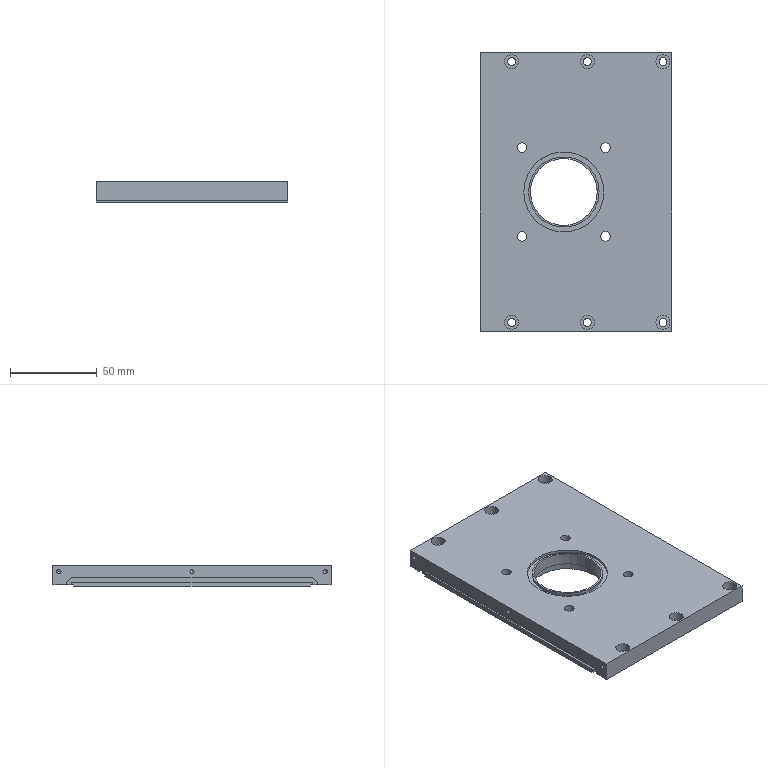NC program | NX | posted with a generic post | part box 110 x 160 x 12 mm
Whole program:
N10 G17 G21 G94 G90
(ZLEVEL_PROFILE_COPY_1_COPY_COPY_1_COPY , TOOL : D10)
N12 T15 M6
N14 G54
N16 G17 G0 G90 X86.926 Y57.566 B0. C0. S9500 M3
N18 G43 Z30. H15
N20 Z0.
N22 G94 G1 Z-1. F1000.
N24 X85.6 Y56.8
N26 G3 X85.1 Y55.934 R1.
N28 G1 Y55.596 F3000.
N30 X85.071 Y55.545
N32 G2 X85.1 Y55. R5.1
N34 G1 Y-55.
N36 G2 X85.071 Y-55.545 R5.1
N38 G1 X85.1 Y-55.596
N40 Y-55.934
N42 G3 X85.6 Y-56.8 R1.
N44 G1 X86.926 Y-57.566
N46 Z0.
N48 G0 Z30.
N50 Z-1.
N52 G1 Z-2. F1000.
N54 X85.6 Y-56.8
N56 G2 X85.1 Y-55.934 R1.
N58 G1 Y-55.596 F3000.
N60 X85.071 Y-55.545
N62 G3 X85.1 Y-55. R5.1
N64 G1 Y55.
N66 G3 X85.071 Y55.545 R5.1
N68 G1 X85.1 Y55.596
N70 Y55.934
N72 G2 X85.6 Y56.8 R1.
N74 G1 X86.926 Y57.566
N76 Z-1.
N78 G0 Z30.
N80 Z-2.
N82 G1 Z-3. F1000.
N84 X85.6 Y56.8
N86 G3 X85.1 Y55.934 R1.
N88 G1 Y55.596 F3000.
N90 X85.071 Y55.545
N92 G2 X85.1 Y55. R5.1
N94 G1 Y-55.
N96 G2 X85.071 Y-55.545 R5.1
N98 G1 X85.1 Y-55.596
N100 Y-55.934
N102 G3 X85.6 Y-56.8 R1.
N104 G1 X86.926 Y-57.566
N106 Z-2.
N108 G0 Z30.
N110 Z-3.
N112 G1 Z-4. F1000.
N114 X85.6 Y-56.8
N116 G2 X85.1 Y-55.934 R1.
N118 G1 Y-55.596 F3000.
N120 X85.071 Y-55.545
N122 G3 X85.1 Y-55. R5.1
N124 G1 Y55.
N126 G3 X85.071 Y55.545 R5.1
N128 G1 X85.1 Y55.596
N130 Y55.934
N132 G2 X85.6 Y56.8 R1.
N134 G1 X86.926 Y57.566
N136 Z-3.
N138 G0 Z30.
N140 Z-4.
N142 G1 Z-5. F1000.
N144 X85.6 Y56.8
N146 G3 X85.1 Y55.934 R1.
N148 G1 Y55.596 F3000.
N150 X85.071 Y55.545
N152 G2 X85.1 Y55. R5.1
N154 G1 Y-55.
N156 G2 X85.071 Y-55.545 R5.1
N158 G1 X85.1 Y-55.596
N160 Y-55.934
N162 G3 X85.6 Y-56.8 R1.
N164 G1 X86.926 Y-57.566
N166 Z-4.
N168 G0 Z30.
N170 Z-5.
N172 G1 Z-6. F1000.
N174 X85.6 Y-56.8
N176 G2 X85.1 Y-55.934 R1.
N178 G1 Y-55.596 F3000.
N180 X85.071 Y-55.545
N182 G3 X85.1 Y-55. R5.1
N184 G1 Y55.
N186 G3 X85.071 Y55.545 R5.1
N188 G1 X85.1 Y55.596
N190 Y55.934
N192 G2 X85.6 Y56.8 R1.
N194 G1 X86.926 Y57.566
N196 Z-5.
N198 G0 Z30.
N200 Z-6.
N202 G1 Z-7. F1000.
N204 X85.6 Y56.8
N206 G3 X85.1 Y55.934 R1.
N208 G1 Y55.596 F3000.
N210 X85.071 Y55.545
N212 G2 X85.1 Y55. R5.1
N214 G1 Y-55.
N216 G2 X85.071 Y-55.545 R5.1
N218 G1 X85.1 Y-55.596
N220 Y-55.934
N222 G3 X85.6 Y-56.8 R1.
N224 G1 X86.926 Y-57.566
N226 Z-6.
N228 G0 Z30.
N230 Z-7.
N232 G1 Z-8. F1000.
N234 X85.6 Y-56.8
N236 G2 X85.1 Y-55.934 R1.
N238 G1 Y-55.596 F3000.
N240 X85.071 Y-55.545
N242 G3 X85.1 Y-55. R5.1
N244 G1 Y55.
N246 G3 X85.071 Y55.545 R5.1
N248 G1 X85.1 Y55.596
N250 Y55.934
N252 G2 X85.6 Y56.8 R1.
N254 G1 X86.926 Y57.566
N256 Z-7.
N258 G0 Z30.
N260 Z-8.
N262 G1 Z-9. F1000.
N264 X85.6 Y56.8
N266 G3 X85.1 Y55.934 R1.
N268 G1 Y55.596 F3000.
N270 X85.071 Y55.545
N272 G2 X85.1 Y55. R5.1
N274 G1 Y-55.
N276 G2 X85.071 Y-55.545 R5.1
N278 G1 X85.1 Y-55.596
N280 Y-55.934
N282 G3 X85.6 Y-56.8 R1.
N284 G1 X86.926 Y-57.566
N286 Z-8.
N288 G0 Z30.
N290 Z-9.
N292 G1 Z-10. F1000.
N294 X85.6 Y-56.8
N296 G2 X85.1 Y-55.934 R1.
N298 G1 Y-55.596 F3000.
N300 X85.071 Y-55.545
N302 G3 X85.1 Y-55. R5.1
N304 G1 Y55.
N306 G3 X85.071 Y55.545 R5.1
N308 G1 X85.1 Y55.596
N310 Y55.934
N312 G2 X85.6 Y56.8 R1.
N314 G1 X86.926 Y57.566
N316 Z-9.
N318 G0 Z30.
N320 Z-10.
N322 G1 Z-11. F1000.
N324 X85.6 Y56.8
N326 G3 X85.1 Y55.934 R1.
N328 G1 Y55.596 F3000.
N330 X85.071 Y55.545
N332 G2 X85.1 Y55. R5.1
N334 G1 Y-55.
N336 G2 X85.071 Y-55.545 R5.1
N338 G1 X85.1 Y-55.596
N340 Y-55.934
N342 G3 X85.6 Y-56.8 R1.
N344 G1 X86.926 Y-57.566
N346 Z-10.
N348 G0 Z30.
N350 Z-11.
N352 G1 Z-12. F1000.
N354 X85.6 Y-56.8
N356 G2 X85.1 Y-55.934 R1.
N358 G1 Y-55.596 F3000.
N360 X85.071 Y-55.545
N362 G3 X85.1 Y-55. R5.1
N364 G1 Y55.
N366 G3 X85.071 Y55.545 R5.1
N368 G1 X85.1 Y55.596
N370 Y55.934
N372 G2 X85.6 Y56.8 R1.
N374 G1 X86.926 Y57.566
N376 Z-11.
N378 G0 Z53.
N380 X-86.924 Y-57.565
N382 Z0.
N384 G1 Z-1. F1000.
N386 X-85.6 Y-56.8
N388 G3 X-85.1 Y-55.934 R1.
N390 G1 Y-54.962 F3000.
N392 Y55.
N394 Y55.934
N396 G3 X-85.6 Y56.8 R1.
N398 G1 X-86.924 Y57.565
N400 Z0.
N402 G0 Z30.
N404 Z-1.
N406 G1 Z-2. F1000.
N408 X-85.6 Y56.8
N410 G2 X-85.1 Y55.934 R1.
N412 G1 Y55. F3000.
N414 Y-54.962
N416 Y-55.934
N418 G2 X-85.6 Y-56.8 R1.
N420 G1 X-86.924 Y-57.565
N422 Z-1.
N424 G0 Z30.
N426 Z-2.
N428 G1 Z-3. F1000.
N430 X-85.6 Y-56.8
N432 G3 X-85.1 Y-55.934 R1.
N434 G1 Y-54.962 F3000.
N436 Y55.
N438 Y55.934
N440 G3 X-85.6 Y56.8 R1.
N442 G1 X-86.924 Y57.565
N444 Z-2.
N446 G0 Z30.
N448 Z-3.
N450 G1 Z-4. F1000.
N452 X-85.6 Y56.8
N454 G2 X-85.1 Y55.934 R1.
N456 G1 Y55. F3000.
N458 Y-54.962
N460 Y-55.934
N462 G2 X-85.6 Y-56.8 R1.
N464 G1 X-86.924 Y-57.565
N466 Z-3.
N468 G0 Z30.
N470 Z-4.
N472 G1 Z-5. F1000.
N474 X-85.6 Y-56.8
N476 G3 X-85.1 Y-55.934 R1.
N478 G1 Y-54.962 F3000.
N480 Y55.
N482 Y55.934
N484 G3 X-85.6 Y56.8 R1.
N486 G1 X-86.924 Y57.565
N488 Z-4.
N490 G0 Z30.
N492 Z-5.
N494 G1 Z-6. F1000.
N496 X-85.6 Y56.8
N498 G2 X-85.1 Y55.934 R1.
N500 G1 Y55. F3000.
N502 Y-54.962
N504 Y-55.934
N506 G2 X-85.6 Y-56.8 R1.
N508 G1 X-86.924 Y-57.565
N510 Z-5.
N512 G0 Z30.
N514 Z-6.
N516 G1 Z-7. F1000.
N518 X-85.6 Y-56.8
N520 G3 X-85.1 Y-55.934 R1.
N522 G1 Y-54.962 F3000.
N524 Y55.
N526 Y55.934
N528 G3 X-85.6 Y56.8 R1.
N530 G1 X-86.924 Y57.565
N532 Z-6.
N534 G0 Z30.
N536 Z-7.
N538 G1 Z-8. F1000.
N540 X-85.6 Y56.8
N542 G2 X-85.1 Y55.934 R1.
N544 G1 Y55. F3000.
N546 Y-54.962
N548 Y-55.934
N550 G2 X-85.6 Y-56.8 R1.
N552 G1 X-86.924 Y-57.565
N554 Z-7.
N556 G0 Z30.
N558 Z-8.
N560 G1 Z-9. F1000.
N562 X-85.6 Y-56.8
N564 G3 X-85.1 Y-55.934 R1.
N566 G1 Y-54.962 F3000.
N568 Y55.
N570 Y55.934
N572 G3 X-85.6 Y56.8 R1.
N574 G1 X-86.924 Y57.565
N576 Z-8.
N578 G0 Z30.
N580 Z-9.
N582 G1 Z-10. F1000.
N584 X-85.6 Y56.8
N586 G2 X-85.1 Y55.934 R1.
N588 G1 Y55. F3000.
N590 Y-54.962
N592 Y-55.934
N594 G2 X-85.6 Y-56.8 R1.
N596 G1 X-86.924 Y-57.565
N598 Z-9.
N600 G0 Z30.
N602 Z-10.
N604 G1 Z-11. F1000.
N606 X-85.6 Y-56.8
N608 G3 X-85.1 Y-55.934 R1.
N610 G1 Y-54.962 F3000.
N612 Y55.
N614 Y55.934
N616 G3 X-85.6 Y56.8 R1.
N618 G1 X-86.924 Y57.565
N620 Z-10.
N622 G0 Z30.
N624 Z-11.
N626 G1 Z-12. F1000.
N628 X-85.6 Y56.8
N630 G2 X-85.1 Y55.934 R1.
N632 G1 Y55. F3000.
N634 Y-54.962
N636 Y-55.934
N638 G2 X-85.6 Y-56.8 R1.
N640 G1 X-86.924 Y-57.565
N642 Z-11.
N644 G0 Z30.
(FLOOR_WALL , TOOL : D10)
N646 X-86.5 Y-1.443
N648 Z0.1
N650 G1 Z-0.9 F1000.
N652 X-85.5 Y-0.866
N654 G3 X-85. Y0. R1.
N656 G1 Y60. F2500.
N658 X-73.1
N660 Y-60.
N662 X-85.
N664 Y0.
N666 X-80.5
N668 Y55.5
N670 X-77.6
N672 Y-55.5
N674 X-80.5
N676 Y0.
N678 G3 X-81. Y0.866 R1.
N680 G1 Z0.1
N682 G0 Z30.
N684 X86.5 Y1.443
N686 Z0.1
N688 G1 Z-0.9 F1000.
N690 X85.5 Y0.866
N692 G3 X85. Y0. R1.
N694 G1 Y-60. F2500.
N696 X73.1
N698 Y60.
N700 X85.
N702 Y0.
N704 X80.5
N706 Y-55.5
N708 X77.6
N710 Y55.5
N712 X80.5
N714 Y0.
N716 G3 X81. Y-0.866 R1.
N718 G1 Z0.1
N720 G0 Z30.
(HOLE_MILLING , TOOL : D10)
N722 X0. Y-7.
N724 Z0.5
N726 G3 X1.25 Y-5.75 R1.25
N728 X0. Y-4.5 R1.25
N730 X0. Y-4.5 Z-0.5 I0. J-2.5
N732 X0. Y-4.5 Z-1.5 I0. J-2.5
N734 X0. Y-4.5 Z-2.5 I0. J-2.5
N736 X0. Y-4.5 Z-3.5 I0. J-2.5
N738 X0. Y-4.5 Z-4.5 I0. J-2.5
N740 X0. Y-9.5 Z-5. I0. J-2.5
N742 X2.678 Y-6.871 R2.679
N744 X0.101 Y-4.007 R2.822
N746 X-3.231 Y-6.769 R3.08
N748 X-0.235 Y-10.481 R3.396
N750 X3.715 Y-7.381 R3.575
N752 X0.402 Y-3.036 R3.891
N754 X-4.191 Y-6.436 R4.071
N756 X-0.601 Y-11.438 R4.386
N758 X4.659 Y-7.779 R4.566
N760 X0.833 Y-2.097 R4.881
N762 X-5.117 Y-5.973 R5.06
N764 X-1.097 Y-12.357 R5.376
N766 X5.563 Y-8.306 R5.555
N768 X1.392 Y-1.202 R5.871
N770 X-5.995 Y-5.384 R6.05
N772 X-1.718 Y-13.224 R6.365
N774 X6.411 Y-8.956 R6.545
N776 X2.074 Y-0.365 R6.86
N778 X-6.812 Y-4.674 R7.04
N780 X-2.459 Y-14.029 R7.355
N782 X7.194 Y-9.725 R7.534
N784 X2.874 Y0.403 R7.85
N786 X-7.556 Y-3.847 R8.029
N788 X-3.315 Y-14.757 R8.344
N790 X7.897 Y-10.607 R8.524
N792 X3.784 Y1.089 R8.839
N794 X-8.216 Y-2.912 R9.019
N796 X-4.279 Y-15.398 R9.334
N798 X8.511 Y-11.594 R9.513
N800 X4.798 Y1.682 R9.829
N802 X-8.78 Y-1.876 R10.008
N804 X-5.341 Y-15.94 R10.323
N806 X9.023 Y-12.678 R10.503
N808 X5.907 Y2.171 R10.818
N810 X-9.238 Y-0.747 R10.997
N812 X-6.494 Y-16.374 R11.313
N814 X9.424 Y-13.849 R11.492
N816 X7.101 Y2.547 R11.807
N818 X-9.58 Y0.464 R11.987
N820 X-7.727 Y-16.689 R12.302
N822 X9.705 Y-15.097 R12.482
N824 X8.37 Y2.8 R12.797
N826 X-9.798 Y1.747 R12.976
N828 X-9.029 Y-16.878 R13.291
N830 X9.857 Y-16.411 R13.471
N832 X9.702 Y2.922 R13.786
N834 X-9.883 Y3.09 R13.966
N836 X-10.388 Y-16.932 R14.281
N838 X9.874 Y-17.78 R14.46
N840 X11.085 Y2.906 R14.776
N842 X-9.829 Y4.48 R14.955
N844 X-11.792 Y-16.844 R15.27
N846 X9.747 Y-19.19 R15.45
N848 X12.506 Y2.746 R15.765
N850 X-9.864 Y5.83 R16.024
N852 X-13.227 Y-16.61 R16.179
N854 X9.61 Y-20.227 R16.35
N856 X-13.227 Y-16.61 R-16.35
N858 X-1.809 Y-18.419 R8.175
N860 X0. Y-7. R8.175
N862 G0 Z30.
(HOLE_MILLING_COPY , TOOL : D10)
N864 Z-4.5
N866 G3 X1.25 Y-5.75 R1.25
N868 X0. Y-4.5 R1.25
N870 X0. Y-4.5 Z-5.5 I0. J-2.5
N872 X0. Y-4.5 Z-6.5 I0. J-2.5
N874 X0. Y-4.5 Z-7.5 I0. J-2.5
N876 X0. Y-4.5 Z-8.5 I0. J-2.5
N878 X0. Y-4.5 Z-9.5 I0. J-2.5
N880 X0. Y-4.5 Z-10.5 I0. J-2.5
N882 X0. Y-4.5 Z-11.5 I0. J-2.5
N884 X0. Y-9.5 Z-12. I0. J-2.5
N886 X2.677 Y-6.971 R2.682
N888 X0.312 Y-4.033 R2.813
N890 X-3.172 Y-6.432 R3.067
N892 X-0.721 Y-10.391 R3.376
N894 X3.563 Y-8.021 R3.55
N896 X1.221 Y-3.243 R3.859
N898 X-3.888 Y-5.439 R4.034
N900 X-1.803 Y-11.05 R4.343
N902 X4.134 Y-9.179 R4.518
N904 X2.458 Y-2.742 R4.827
N906 X-4.29 Y-4.138 R5.001
N908 X-3.174 Y-11.369 R5.31
N910 X4.343 Y-10.599 R5.485
N912 X3.937 Y-2.628 R5.794
N914 X-4.285 Y-2.625 R5.969
N916 X-4.731 Y-11.26 R6.277
N918 X4.108 Y-12.175 R6.452
N920 X5.542 Y-2.974 R6.761
N922 X-3.808 Y-1.019 R6.935
N924 X-6.351 Y-10.667 R7.244
N926 X3.381 Y-13.777 R7.419
N928 X7.141 Y-3.821 R7.728
N930 X-2.828 Y0.545 R7.902
N932 X-7.894 Y-9.565 R8.211
N934 X2.149 Y-15.266 R8.386
N936 X8.591 Y-5.174 R8.695
N938 X-1.349 Y1.923 R8.869
N940 X-9.216 Y-7.969 R9.178
N942 X0.434 Y-16.498 R9.353
N944 X9.75 Y-7. R9.661
N946 X0.587 Y2.974 R9.836
N948 X-10.177 Y-5.93 R10.145
N950 X-1.701 Y-17.335 R10.319
N952 X10.482 Y-9.228 R10.628
N954 X2.898 Y3.568 R10.803
N956 X-10.652 Y-3.539 R11.112
N958 X-4.16 Y-17.658 R11.286
N960 X10.673 Y-11.752 R11.595
N962 X5.47 Y3.596 R11.77
N964 X-10.537 Y-0.917 R12.078
N966 X-6.811 Y-17.371 R12.253
N968 X10.234 Y-14.435 R12.562
N970 X8.162 Y2.978 R12.736
N972 X-9.76 Y1.788 R13.045
N974 X-9.502 Y-16.412 R13.22
N976 X9.111 Y-17.119 R13.528
N978 X10.728 Y1.895 R13.783
N980 X-8.288 Y4.407 R13.926
N982 X-11.407 Y-15.288 R14.1
N984 X-8.288 Y4.407 R-14.1
N986 X-9.847 Y-5.44 R7.05
N988 X0. Y-7. R7.05
N990 G0 Z30.
N992 M5
(ZLEVEL_PROFILE_COPY_1_COPY_COPY_1 , TOOL : D10JING)
N994 T14 M6
N996 G54
N998 G17 G0 G90 X86.925 Y61.48 B0. C0. S9500 M3
N1000 G43 Z30. H14
N1002 Z-11.
N1004 G94 G1 Z-12. F1000.
N1006 X85.5 Y60.657
N1008 G3 X85. Y59.791 R1.
N1010 G1 Y52.317 F1200.
N1012 Y-55.
N1014 G2 X84.975 Y-55.497 R5.
N1016 G1 X85. Y-55.548
N1018 Y-59.791
N1020 G3 X85.5 Y-60.657 R1.
N1022 G1 X86.93 Y-61.483
N1024 Z-11.
N1026 G0 Z30.
N1028 X-86.925 Y-61.48
N1030 Z-11.
N1032 G1 Z-12. F1000.
N1034 X-85.5 Y-60.657
N1036 G3 X-85. Y-59.791 R1.
N1038 G1 Y-54.962 F1200.
N1040 Y52.317
N1042 Y59.791
N1044 G3 X-85.5 Y60.657 R1.
N1046 G1 X-86.93 Y61.483
N1048 Z-11.
N1050 G0 Z30.
(ZLEVEL_PROFILE_COPY_1_COPY_COPY_1_COPY_1 , TOOL : D10JING)
N1052 X-1.797 Y-21.388
N1054 Z-4.
N1056 G1 Z-5. F1000.
N1058 X-0.866 Y-23.
N1060 G3 X0. Y-23.5 R1.
N1062 X16.5 Y-7. R16.5 F1200.
N1064 X0. Y-23.5 R-16.5
N1066 X0.866 Y-23. R1.
N1068 G1 X1.797 Y-21.388
N1070 Z-4.
N1072 G0 Z30.
(ZLEVEL_PROFILE_COPY_1_COPY_COPY_1_COPY_1_COPY , TOOL : D10JING)
N1074 X-7.555 Y-16.643
N1076 Z-11.
N1078 G1 Z-12. F1000.
N1080 X-7.538 Y-18.534
N1082 G3 X-7.03 Y-19.395 R1.
N1084 G1 X-6.993 Y-19.416 F1200.
N1086 G3 X10.042 Y-17.111 R14.25
N1088 G1 X10.046 Y-17.086
N1090 X10.054 Y-17.034
N1092 X10.105 Y-17.047
N1094 G3 X10.846 Y-16.242 R14.25
N1096 G1 X10.842 Y-16.21
N1098 X10.878 Y-16.205
N1100 G3 X13.176 Y-12.428 R14.25
N1102 G1 X13.165 Y-12.4
N1104 X13.423 Y-11.712
N1106 X13.462 Y-11.673
N1108 G3 X12.423 Y-0.019 R14.25
N1110 G1 X12.39 Y-0.015
N1112 X12.403 Y0.016
N1114 G3 X11.642 Y1.218 R14.25
N1116 G1 X11.392 Y1.518
N1118 X11.395 Y1.556
N1120 G3 X9.314 Y3.785 R14.25
N1122 G1 X9.208 Y3.842
N1124 X9.203 Y3.88
N1126 G3 X7.019 Y5.402 R14.25
N1128 G1 X6.988 Y5.39
N1130 X6.981 Y5.423
N1132 G3 X5.409 Y6.183 R14.25
N1134 G1 X5.381 Y6.165
N1136 X5.37 Y6.199
N1138 G3 X-5.37 Y6.199 R14.25
N1140 G1 X-5.381 Y6.165
N1142 X-5.409 Y6.183
N1144 G3 X-6.981 Y5.423 R14.25
N1146 G1 X-6.988 Y5.39
N1148 X-7.019 Y5.402
N1150 G3 X-9.203 Y3.88 R14.25
N1152 G1 X-9.208 Y3.842
N1154 X-9.315 Y3.784
N1156 G3 X-11.395 Y1.556 R14.25
N1158 G1 X-11.392 Y1.518
N1160 X-11.642 Y1.218
N1162 G3 X-12.403 Y0.016 R14.25
N1164 G1 X-12.39 Y-0.015
N1166 X-12.423 Y-0.019
N1168 G3 X-10.879 Y-16.203 R14.25
N1170 G1 X-10.842 Y-16.21
N1172 X-10.846 Y-16.242
N1174 G3 X-10.11 Y-17.043 R14.25
N1176 G1 X-10.067 Y-17.051
N1178 X-10.025 Y-17.067
N1180 X-10.046 Y-17.107
N1182 G3 X-7.03 Y-19.395 R14.25
N1184 X-6.03 Y-19.388 R1.
N1186 G1 X-4.403 Y-18.432
N1188 Z-11.
N1190 G0 Z30.
(FLOOR_WALL_1 , TOOL : D10JING)
N1192 X-85.975 Y-61.14
N1194 Z0.5
N1196 G1 Z-1. F1250.
N1198 X-85.5 Y-60.866
N1200 G3 X-85. Y-60. R1.
N1202 G1 Y60.
N1204 X-81.167
N1206 Y-60.
N1208 X-77.333
N1210 Y60.
N1212 X-73.5
N1214 Y-60.
N1216 G2 X-74. Y-60.866 R1.
N1218 G1 X-75.098 Y-61.5
N1220 Z0.5
N1222 G0 Z30.
N1224 X-74.598
N1226 Z0.5
N1228 G1 Z-1.
N1230 X-73.5 Y-60.866
N1232 G3 X-73. Y-60. R1.
N1234 G1 Y60.
N1236 G3 X-73.5 Y60.866 R1.
N1238 G1 X-74.598 Y61.5
N1240 Z0.5
N1242 G0 Z30.
N1244 X85.975 Y61.14
N1246 Z0.5
N1248 G1 Z-1.
N1250 X85.5 Y60.866
N1252 G3 X85. Y60. R1.
N1254 G1 Y-60.
N1256 X81.167
N1258 Y60.
N1260 X77.333
N1262 Y-60.
N1264 X73.5
N1266 Y60.
N1268 G2 X74. Y60.866 R1.
N1270 G1 X75.098 Y61.5
N1272 Z0.5
N1274 G0 Z30.
N1276 X74.598
N1278 Z0.5
N1280 G1 Z-1.
N1282 X73.5 Y60.866
N1284 G3 X73. Y60. R1.
N1286 G1 Y-60.
N1288 G3 X73.5 Y-60.866 R1.
N1290 G1 X74.598 Y-61.5
N1292 Z0.5
N1294 G0 Z30.
N1296 M5
(DRILLING_COPY_1 , TOOL : D6A45)
N1298 T01 M6
N1300 G54
N1302 G17 G0 G90 X75. Y50. B0. C0. S5000 M3
N1304 G43 Z30. H1
N1306 G94 G81 G98 Z-2. F350. R2.
N1308 Y6.5
N1310 Y-37.
N1312 X25.5 Y-31. Z-1. R3.
N1314 Y17.
N1316 X0. Y-7.
N1318 X-25.5 Y17.
N1320 Y-31.
N1322 X-75. Y-37. Z-2. R2.
N1324 Y6.5
N1326 Y50.
N1328 G80
N1330 G0 X-75. Y50. Z30.
N1332 M5
(DRILLING_COPY_1_COPY_COPY , TOOL : 4.5ZT)
N1334 T08 M6
N1336 G54
N1338 G17 G0 G90 X-75. Y-37. B0. C0. S2000 M3
N1340 G43 Z30. H8
N1342 G94 G83 G98 Z-9.852 F200. Q2. R2.
N1344 Y6.5
N1346 Y50.
N1348 X75.
N1350 Y6.5
N1352 Y-37.
N1354 G80
N1356 G0 X75. Y-37. Z30.
N1358 M5
(DRILLING_COPY_1_COPY_COPY_COPY , TOOL : 5.5ZT)
N1360 T09 M6
N1362 G54
N1364 G17 G0 G90 X25.5 Y-31. B0. C0. S2000 M3
N1366 G43 Z30. H9
N1368 G94 G83 G98 Z-15.152 F200. Q2. R3.
N1370 Y17.
N1372 X-25.5
N1374 Y-31.
N1376 G80
N1378 G0 X-25.5 Y-31. Z30.
N1380 M5
(PLANAR_MILL_COPY_COPY_COPY_COPY_COPY_COPY_1 , TOOL : D6A45)
N1382 T01 M6
N1384 G54
N1386 G17 G0 G90 X-24.634 Y18.69 B0. C0. S9500 M3
N1388 G43 Z30. H1
N1390 Z0.84
N1392 G94 G1 Z-0.66 F1250.
N1394 G3 X-25.5 Y19.19 R1.
N1396 X-27.69 Y17. R2.19
N1398 X-25.5 Y19.19 R-2.19
N1400 X-26.366 Y18.69 R1.
N1402 G1 Z0.84
N1404 G0 Z30.
N1406 X-0.866 Y56.06
N1408 Z0.84
N1410 G1 Z-0.66
N1412 G3 X0. Y55.56 R1.
N1414 G1 X68.
N1416 G2 X68.56 Y55. R0.56
N1418 G1 Y-55.
N1420 G2 X68. Y-55.56 R0.56
N1422 G1 X-68.
N1424 G2 X-68.56 Y-55. R0.56
N1426 G1 Y55.
N1428 G2 X-68. Y55.56 R0.56
N1430 G1 X0.
N1432 G3 X0.866 Y56.06 R1.
N1434 G1 Z0.84
N1436 G0 Z30.
N1438 X26.366 Y18.69
N1440 Z0.84
N1442 G1 Z-0.66
N1444 G3 X25.5 Y19.19 R1.
N1446 X23.31 Y17. R2.19
N1448 X25.5 Y19.19 R-2.19
N1450 X24.634 Y18.69 R1.
N1452 G1 Z0.84
N1454 G0 Z30.
N1456 Y-32.69
N1458 Z0.84
N1460 G1 Z-0.66
N1462 G3 X25.5 Y-33.19 R1.
N1464 X27.69 Y-31. R2.19
N1466 X25.5 Y-33.19 R-2.19
N1468 X26.366 Y-32.69 R1.
N1470 G1 Z0.84
N1472 G0 Z30.
N1474 X-0.866 Y-27.44
N1476 Z0.84
N1478 G1 Z-0.66
N1480 G3 X0. Y-27.94 R1.
N1482 X20.94 Y-7. R20.94
N1484 X0. Y-27.94 R-20.94
N1486 X0.866 Y-27.44 R1.
N1488 G1 Z0.84
N1490 G0 Z30.
N1492 X-26.366 Y-32.69
N1494 Z0.84
N1496 G1 Z-0.66
N1498 G3 X-25.5 Y-33.19 R1.
N1500 X-23.31 Y-31. R2.19
N1502 X-25.5 Y-33.19 R-2.19
N1504 X-24.634 Y-32.69 R1.
N1506 G1 Z0.84
N1508 G0 Z30.
(PLANAR_MILL_COPY_COPY_COPY_COPY_COPY_COPY_1_COPY , TOOL : D6A45)
N1510 X75.105 Y49.893
N1512 Z-0.5
N1514 G1 Z-2.
N1516 X75.85 Y49.134
N1518 G3 X76.35 Y50. R1.
N1520 X75. Y51.35 R1.35
N1522 X76.35 Y50. R-1.35
N1524 X75.85 Y50.866 R1.
N1526 G1 X75.105 Y50.107
N1528 Z-0.5
N1530 G0 Z30.
N1532 Y6.393
N1534 Z-0.5
N1536 G1 Z-2.
N1538 X75.85 Y5.634
N1540 G3 X76.35 Y6.5 R1.
N1542 X75. Y7.85 R1.35
N1544 X76.35 Y6.5 R-1.35
N1546 X75.85 Y7.366 R1.
N1548 G1 X75.105 Y6.607
N1550 Z-0.5
N1552 G0 Z30.
N1554 Y-37.107
N1556 Z-0.5
N1558 G1 Z-2.
N1560 X75.85 Y-37.866
N1562 G3 X76.35 Y-37. R1.
N1564 X75. Y-35.65 R1.35
N1566 X76.35 Y-37. R-1.35
N1568 X75.85 Y-36.134 R1.
N1570 G1 X75.105 Y-36.893
N1572 Z-0.5
N1574 G0 Z30.
N1576 X74.304 Y57.269
N1578 Z-0.5
N1580 G1 Z-2.
N1582 X73.777 Y56.836
N1584 G3 X73.426 Y55.9 R1.
N1586 G1 X79.9
N1588 G2 X80.9 Y54.9 R1.
N1590 G1 Y-54.9
N1592 G2 X79.9 Y-55.9 R1.
N1594 G1 X73.426
N1596 G3 X73.777 Y-56.836 R1.
N1598 G1 X74.304 Y-57.269
N1600 Z-0.5
N1602 G0 Z30.
N1604 X-74.304
N1606 Z-0.5
N1608 G1 Z-2.
N1610 X-73.777 Y-56.836
N1612 G3 X-73.426 Y-55.9 R1.
N1614 G1 X-79.9
N1616 G2 X-80.9 Y-54.9 R1.
N1618 G1 Y54.9
N1620 G2 X-79.9 Y55.9 R1.
N1622 G1 X-73.426
N1624 G3 X-73.777 Y56.836 R1.
N1626 G1 X-74.304 Y57.269
N1628 Z-0.5
N1630 G0 Z30.
N1632 X-75.105 Y-36.893
N1634 Z-0.5
N1636 G1 Z-2.
N1638 X-75.85 Y-36.134
N1640 G3 X-76.35 Y-37. R1.
N1642 X-75. Y-38.35 R1.35
N1644 X-76.35 Y-37. R-1.35
N1646 X-75.85 Y-37.866 R1.
N1648 G1 X-75.105 Y-37.107
N1650 Z-0.5
N1652 G0 Z30.
N1654 Y6.607
N1656 Z-0.5
N1658 G1 Z-2.
N1660 X-75.85 Y7.366
N1662 G3 X-76.35 Y6.5 R1.
N1664 X-75. Y5.15 R1.35
N1666 X-76.35 Y6.5 R-1.35
N1668 X-75.85 Y5.634 R1.
N1670 G1 X-75.105 Y6.393
N1672 Z-0.5
N1674 G0 Z30.
N1676 Y50.107
N1678 Z-0.5
N1680 G1 Z-2.
N1682 X-75.85 Y50.866
N1684 G3 X-76.35 Y50. R1.
N1686 X-75. Y48.65 R1.35
N1688 X-76.35 Y50. R-1.35
N1690 X-75.85 Y49.134 R1.
N1692 G1 X-75.105 Y49.893
N1694 Z-0.5
N1696 G0 Z30.
N1698 M5
N1700 M2